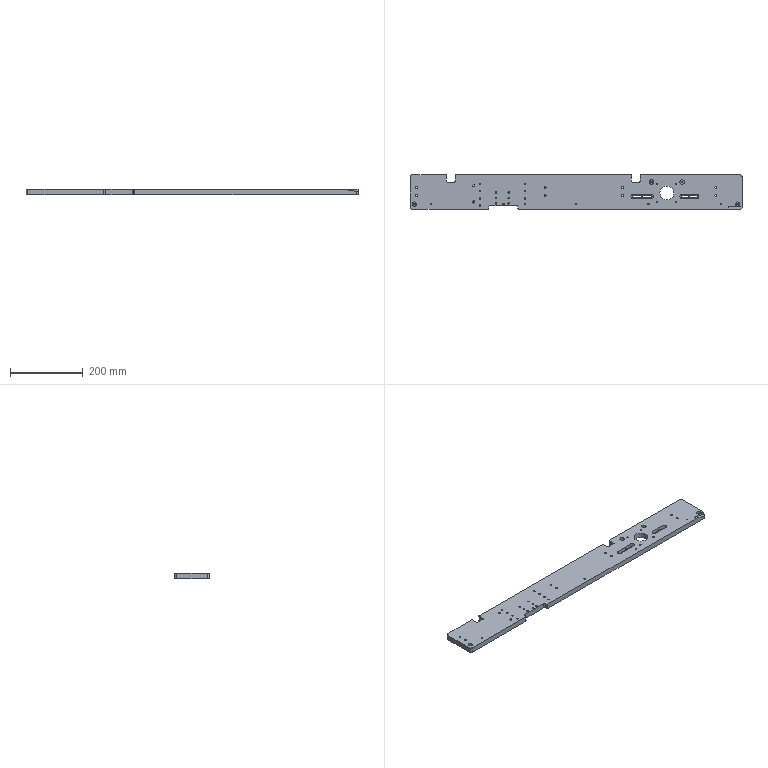Part | STEP file | 1-S938U-100524-004 | 3 solids | 107 faces | box 915 x 95 x 15 mm | volume 1230694 mm3 | cylinder 69 | plane 38 | commonest cylinder face diameters 4.134 x23 4 x8 4.4 x8 4.917 x8 6 x4 10 x4